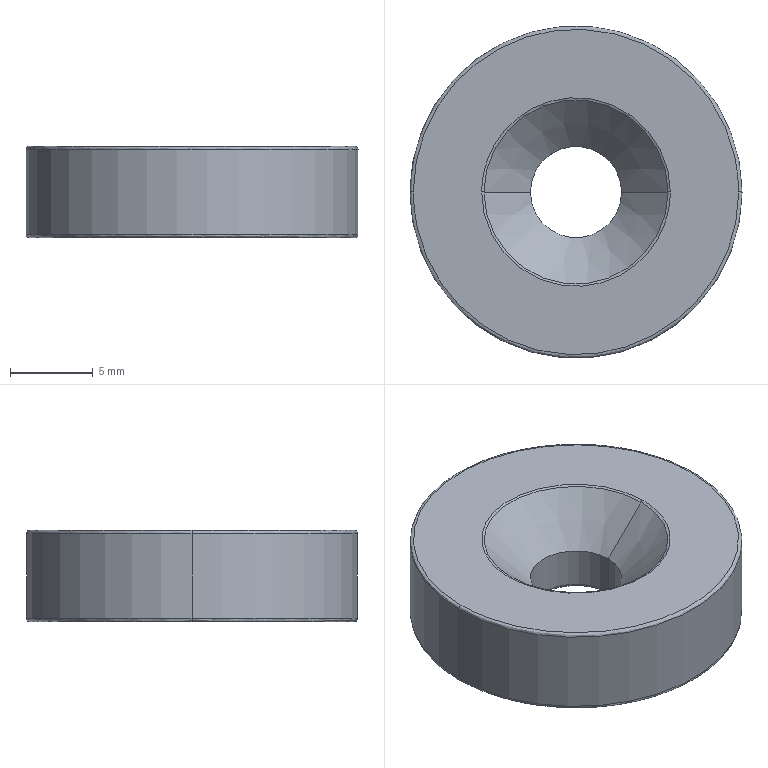Part | STEP file | NHXCC20-5.5 | 1 solid | 16 faces | box 20 x 20 x 5.5 mm | volume 1502 mm3 | spline 8 | cylinder 4 | cone 2 | plane 2 | commonest cylinder face diameters 5.5 x2 20 x2